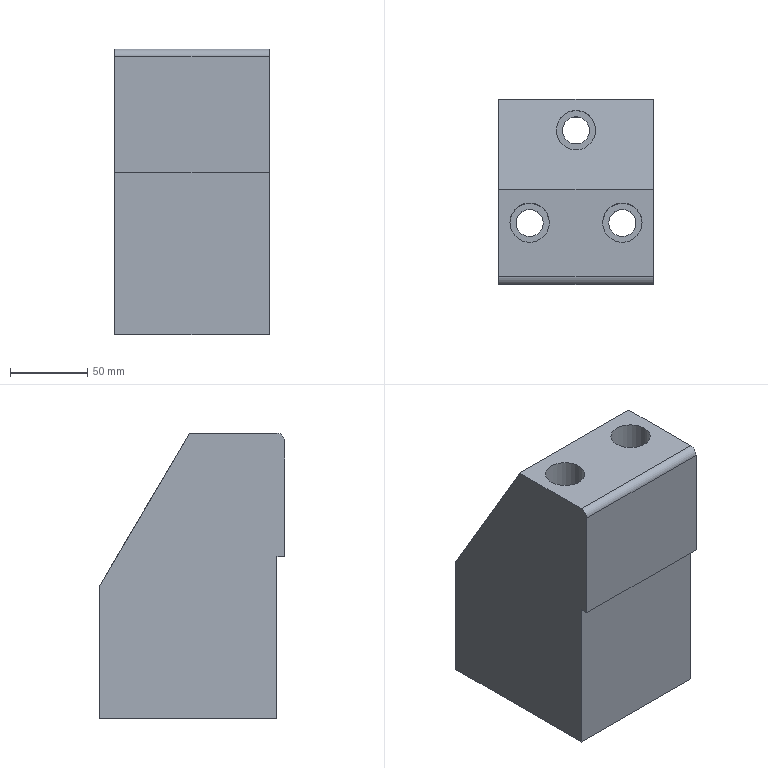Part | NX | features solid 2 | 1 solid | 19 faces | box 100 x 120 x 185 mm | volume 1651296 mm3 | plane 12 | cylinder 7 | commonest cylinder face diameters 17.5 x3 25.5 x3 10 x1
STEP:
#1=CARTESIAN_POINT('',(-412.5,235.,5.));
#2=VERTEX_POINT('',#1);
#3=CARTESIAN_POINT('',(-412.5,291.602,5.));
#4=VERTEX_POINT('',#3);
#5=CARTESIAN_POINT('',(-412.5,230.,5.));
#6=DIRECTION('',(0.,1.,0.));
#7=VECTOR('',#6,1000.);
#8=LINE('',#5,#7);
#9=EDGE_CURVE('',#2,#4,#8,.T.);
#10=ORIENTED_EDGE('',*,*,#9,.F.);
#11=CARTESIAN_POINT('',(-412.5,230.,0.));
#12=VERTEX_POINT('',#11);
#13=CARTESIAN_POINT('',(-412.5,235.,0.));
#14=DIRECTION('',(-1.,0.,0.));
#15=DIRECTION('',(0.,0.,1.));
#16=AXIS2_PLACEMENT_3D('',#13,#14,#15);
#17=CIRCLE('',#16,5.);
#18=EDGE_CURVE('',#2,#12,#17,.F.);
#19=ORIENTED_EDGE('',*,*,#18,.T.);
#20=CARTESIAN_POINT('',(-412.5,230.,-75.));
#21=VERTEX_POINT('',#20);
#22=CARTESIAN_POINT('',(-412.5,230.,-75.));
#23=DIRECTION('',(0.,0.,1.));
#24=VECTOR('',#23,1000.);
#25=LINE('',#22,#24);
#26=EDGE_CURVE('',#21,#12,#25,.T.);
#27=ORIENTED_EDGE('',*,*,#26,.F.);
#28=CARTESIAN_POINT('',(-412.5,235.,-75.));
#29=VERTEX_POINT('',#28);
#30=CARTESIAN_POINT('',(-412.5,230.,-75.));
#31=DIRECTION('',(0.,-1.,0.));
#32=VECTOR('',#31,1000.);
#33=LINE('',#30,#32);
#34=EDGE_CURVE('',#21,#29,#33,.F.);
#35=ORIENTED_EDGE('',*,*,#34,.T.);
#36=CARTESIAN_POINT('',(-412.5,235.,-180.));
#37=VERTEX_POINT('',#36);
#38=CARTESIAN_POINT('',(-412.5,235.,-75.));
#39=DIRECTION('',(0.,0.,-1.));
#40=VECTOR('',#39,1000.);
#41=LINE('',#38,#40);
#42=EDGE_CURVE('',#29,#37,#41,.T.);
#43=ORIENTED_EDGE('',*,*,#42,.T.);
#44=CARTESIAN_POINT('',(-412.5,350.,-180.));
#45=VERTEX_POINT('',#44);
#46=CARTESIAN_POINT('',(-412.5,230.,-180.));
#47=DIRECTION('',(0.,1.,0.));
#48=VECTOR('',#47,1000.);
#49=LINE('',#46,#48);
#50=EDGE_CURVE('',#37,#45,#49,.T.);
#51=ORIENTED_EDGE('',*,*,#50,.T.);
#52=CARTESIAN_POINT('',(-412.5,350.,-94.277));
#53=VERTEX_POINT('',#52);
#54=CARTESIAN_POINT('',(-412.5,350.,-75.));
#55=DIRECTION('',(0.,0.,1.));
#56=VECTOR('',#55,1000.);
#57=LINE('',#54,#56);
#58=EDGE_CURVE('',#45,#53,#57,.T.);
#59=ORIENTED_EDGE('',*,*,#58,.T.);
#60=CARTESIAN_POINT('',(-412.5,310.727,-27.513));
#61=DIRECTION('',(0.,-0.507,0.8619));
#62=VECTOR('',#61,1000.);
#63=LINE('',#60,#62);
#64=EDGE_CURVE('',#53,#4,#63,.T.);
#65=ORIENTED_EDGE('',*,*,#64,.T.);
#66=EDGE_LOOP('',(#10,#19,#27,#35,#43,#51,#59,#65));
#67=FACE_BOUND('',#66,.T.);
#68=CARTESIAN_POINT('',(-412.5,230.,-75.));
#69=DIRECTION('',(-1.,0.,0.));
#70=DIRECTION('',(0.,0.,1.));
#71=AXIS2_PLACEMENT_3D('',#68,#69,#70);
#72=PLANE('',#71);
#73=ADVANCED_FACE('',(#67),#72,.F.);
#74=CARTESIAN_POINT('',(-423.75,270.,-180.));
#75=VERTEX_POINT('',#74);
#76=CARTESIAN_POINT('',(-432.5,270.,-180.));
#77=DIRECTION('',(0.,0.,1.));
#78=DIRECTION('',(1.,0.,0.));
#79=AXIS2_PLACEMENT_3D('',#76,#77,#78);
#80=CIRCLE('',#79,8.75);
#81=EDGE_CURVE('',#75,#75,#80,.T.);
#82=ORIENTED_EDGE('',*,*,#81,.T.);
#83=EDGE_LOOP('',(#82));
#84=FACE_BOUND('',#83,.T.);
#85=CARTESIAN_POINT('',(-483.75,270.,-180.));
#86=VERTEX_POINT('',#85);
#87=CARTESIAN_POINT('',(-492.5,270.,-180.));
#88=DIRECTION('',(0.,0.,1.));
#89=DIRECTION('',(1.,0.,0.));
#90=AXIS2_PLACEMENT_3D('',#87,#88,#89);
#91=CIRCLE('',#90,8.75);
#92=EDGE_CURVE('',#86,#86,#91,.T.);
#93=ORIENTED_EDGE('',*,*,#92,.T.);
#94=EDGE_LOOP('',(#93));
#95=FACE_BOUND('',#94,.T.);
#96=CARTESIAN_POINT('',(-453.75,330.,-180.));
#97=VERTEX_POINT('',#96);
#98=CARTESIAN_POINT('',(-462.5,330.,-180.));
#99=DIRECTION('',(0.,0.,1.));
#100=DIRECTION('',(1.,0.,0.));
#101=AXIS2_PLACEMENT_3D('',#98,#99,#100);
#102=CIRCLE('',#101,8.75);
#103=EDGE_CURVE('',#97,#97,#102,.T.);
#104=ORIENTED_EDGE('',*,*,#103,.T.);
#105=EDGE_LOOP('',(#104));
#106=FACE_BOUND('',#105,.T.);
#107=CARTESIAN_POINT('',(-512.5,235.,-180.));
#108=VERTEX_POINT('',#107);
#109=CARTESIAN_POINT('',(-487.5,235.,-180.));
#110=DIRECTION('',(1.,0.,0.));
#111=VECTOR('',#110,1000.);
#112=LINE('',#109,#111);
#113=EDGE_CURVE('',#108,#37,#112,.T.);
#114=ORIENTED_EDGE('',*,*,#113,.F.);
#115=CARTESIAN_POINT('',(-512.5,350.,-180.));
#116=VERTEX_POINT('',#115);
#117=CARTESIAN_POINT('',(-512.5,230.,-180.));
#118=DIRECTION('',(0.,1.,0.));
#119=VECTOR('',#118,1000.);
#120=LINE('',#117,#119);
#121=EDGE_CURVE('',#108,#116,#120,.T.);
#122=ORIENTED_EDGE('',*,*,#121,.T.);
#123=CARTESIAN_POINT('',(-487.5,350.,-180.));
#124=DIRECTION('',(1.,0.,0.));
#125=VECTOR('',#124,1000.);
#126=LINE('',#123,#125);
#127=EDGE_CURVE('',#116,#45,#126,.T.);
#128=ORIENTED_EDGE('',*,*,#127,.T.);
#129=ORIENTED_EDGE('',*,*,#50,.F.);
#130=EDGE_LOOP('',(#114,#122,#128,#129));
#131=FACE_BOUND('',#130,.T.);
#132=CARTESIAN_POINT('',(-487.5,230.,-180.));
#133=DIRECTION('',(0.,0.,1.));
#134=DIRECTION('',(1.,0.,0.));
#135=AXIS2_PLACEMENT_3D('',#132,#133,#134);
#136=PLANE('',#135);
#137=ADVANCED_FACE('',(#84,#95,#106,#131),#136,.F.);
#138=CARTESIAN_POINT('',(-512.5,230.,0.));
#139=VERTEX_POINT('',#138);
#140=CARTESIAN_POINT('',(-512.5,230.,-75.));
#141=VERTEX_POINT('',#140);
#142=CARTESIAN_POINT('',(-512.5,230.,25.));
#143=DIRECTION('',(0.,0.,1.));
#144=VECTOR('',#143,1000.);
#145=LINE('',#142,#144);
#146=EDGE_CURVE('',#139,#141,#145,.F.);
#147=ORIENTED_EDGE('',*,*,#146,.F.);
#148=CARTESIAN_POINT('',(-512.5,235.,5.));
#149=VERTEX_POINT('',#148);
#150=CARTESIAN_POINT('',(-512.5,235.,0.));
#151=DIRECTION('',(1.,0.,0.));
#152=DIRECTION('',(0.,0.,-1.));
#153=AXIS2_PLACEMENT_3D('',#150,#151,#152);
#154=CIRCLE('',#153,5.);
#155=EDGE_CURVE('',#139,#149,#154,.F.);
#156=ORIENTED_EDGE('',*,*,#155,.T.);
#157=CARTESIAN_POINT('',(-512.5,291.602,5.));
#158=VERTEX_POINT('',#157);
#159=CARTESIAN_POINT('',(-512.5,230.,5.));
#160=DIRECTION('',(0.,1.,0.));
#161=VECTOR('',#160,1000.);
#162=LINE('',#159,#161);
#163=EDGE_CURVE('',#149,#158,#162,.T.);
#164=ORIENTED_EDGE('',*,*,#163,.T.);
#165=CARTESIAN_POINT('',(-512.5,350.,-94.277));
#166=VERTEX_POINT('',#165);
#167=CARTESIAN_POINT('',(-512.5,267.026,46.78));
#168=DIRECTION('',(0.,0.507,-0.8619));
#169=VECTOR('',#168,1000.);
#170=LINE('',#167,#169);
#171=EDGE_CURVE('',#158,#166,#170,.T.);
#172=ORIENTED_EDGE('',*,*,#171,.T.);
#173=CARTESIAN_POINT('',(-512.5,350.,25.));
#174=DIRECTION('',(0.,0.,-1.));
#175=VECTOR('',#174,1000.);
#176=LINE('',#173,#175);
#177=EDGE_CURVE('',#166,#116,#176,.T.);
#178=ORIENTED_EDGE('',*,*,#177,.T.);
#179=ORIENTED_EDGE('',*,*,#121,.F.);
#180=CARTESIAN_POINT('',(-512.5,235.,-75.));
#181=VERTEX_POINT('',#180);
#182=CARTESIAN_POINT('',(-512.5,235.,-75.));
#183=DIRECTION('',(0.,0.,-1.));
#184=VECTOR('',#183,1000.);
#185=LINE('',#182,#184);
#186=EDGE_CURVE('',#181,#108,#185,.T.);
#187=ORIENTED_EDGE('',*,*,#186,.F.);
#188=CARTESIAN_POINT('',(-512.5,230.,-75.));
#189=DIRECTION('',(0.,-1.,0.));
#190=VECTOR('',#189,1000.);
#191=LINE('',#188,#190);
#192=EDGE_CURVE('',#141,#181,#191,.F.);
#193=ORIENTED_EDGE('',*,*,#192,.F.);
#194=EDGE_LOOP('',(#147,#156,#164,#172,#178,#179,#187,#193));
#195=FACE_BOUND('',#194,.T.);
#196=CARTESIAN_POINT('',(-512.5,230.,25.));
#197=DIRECTION('',(1.,0.,0.));
#198=DIRECTION('',(0.,0.,-1.));
#199=AXIS2_PLACEMENT_3D('',#196,#197,#198);
#200=PLANE('',#199);
#201=ADVANCED_FACE('',(#195),#200,.F.);
#202=ORIENTED_EDGE('',*,*,#26,.T.);
#203=CARTESIAN_POINT('',(-512.5,230.,0.));
#204=DIRECTION('',(-1.,0.,0.));
#205=VECTOR('',#204,1000.);
#206=LINE('',#203,#205);
#207=EDGE_CURVE('',#12,#139,#206,.T.);
#208=ORIENTED_EDGE('',*,*,#207,.T.);
#209=ORIENTED_EDGE('',*,*,#146,.T.);
#210=CARTESIAN_POINT('',(-487.5,230.,-75.));
#211=DIRECTION('',(-1.,0.,0.));
#212=VECTOR('',#211,1000.);
#213=LINE('',#210,#212);
#214=EDGE_CURVE('',#141,#21,#213,.F.);
#215=ORIENTED_EDGE('',*,*,#214,.T.);
#216=EDGE_LOOP('',(#202,#208,#209,#215));
#217=FACE_BOUND('',#216,.T.);
#218=CARTESIAN_POINT('',(-487.5,230.,25.));
#219=DIRECTION('',(0.,-1.,0.));
#220=DIRECTION('',(1.,0.,0.));
#221=AXIS2_PLACEMENT_3D('',#218,#219,#220);
#222=PLANE('',#221);
#223=ADVANCED_FACE('',(#217),#222,.T.);
#224=CARTESIAN_POINT('',(-445.25,270.,5.));
#225=VERTEX_POINT('',#224);
#226=CARTESIAN_POINT('',(-432.5,270.,5.));
#227=DIRECTION('',(0.,0.,-1.));
#228=DIRECTION('',(-1.,0.,0.));
#229=AXIS2_PLACEMENT_3D('',#226,#227,#228);
#230=CIRCLE('',#229,12.75);
#231=EDGE_CURVE('',#225,#225,#230,.T.);
#232=ORIENTED_EDGE('',*,*,#231,.T.);
#233=EDGE_LOOP('',(#232));
#234=FACE_BOUND('',#233,.T.);
#235=CARTESIAN_POINT('',(-505.25,270.,5.));
#236=VERTEX_POINT('',#235);
#237=CARTESIAN_POINT('',(-492.5,270.,5.));
#238=DIRECTION('',(0.,0.,-1.));
#239=DIRECTION('',(-1.,0.,0.));
#240=AXIS2_PLACEMENT_3D('',#237,#238,#239);
#241=CIRCLE('',#240,12.75);
#242=EDGE_CURVE('',#236,#236,#241,.T.);
#243=ORIENTED_EDGE('',*,*,#242,.T.);
#244=EDGE_LOOP('',(#243));
#245=FACE_BOUND('',#244,.T.);
#246=ORIENTED_EDGE('',*,*,#163,.F.);
#247=CARTESIAN_POINT('',(-412.5,235.,5.));
#248=DIRECTION('',(-1.,0.,0.));
#249=VECTOR('',#248,1000.);
#250=LINE('',#247,#249);
#251=EDGE_CURVE('',#149,#2,#250,.F.);
#252=ORIENTED_EDGE('',*,*,#251,.T.);
#253=ORIENTED_EDGE('',*,*,#9,.T.);
#254=CARTESIAN_POINT('',(-412.5,291.602,5.));
#255=DIRECTION('',(-1.,0.,0.));
#256=VECTOR('',#255,1000.);
#257=LINE('',#254,#256);
#258=EDGE_CURVE('',#4,#158,#257,.T.);
#259=ORIENTED_EDGE('',*,*,#258,.T.);
#260=EDGE_LOOP('',(#246,#252,#253,#259));
#261=FACE_BOUND('',#260,.T.);
#262=CARTESIAN_POINT('',(-412.5,230.,5.));
#263=DIRECTION('',(0.,0.,-1.));
#264=DIRECTION('',(-1.,0.,0.));
#265=AXIS2_PLACEMENT_3D('',#262,#263,#264);
#266=PLANE('',#265);
#267=ADVANCED_FACE('',(#234,#245,#261),#266,.F.);
#268=ORIENTED_EDGE('',*,*,#177,.F.);
#269=CARTESIAN_POINT('',(-487.5,350.,-94.277));
#270=DIRECTION('',(1.,0.,0.));
#271=VECTOR('',#270,1000.);
#272=LINE('',#269,#271);
#273=EDGE_CURVE('',#166,#53,#272,.T.);
#274=ORIENTED_EDGE('',*,*,#273,.T.);
#275=ORIENTED_EDGE('',*,*,#58,.F.);
#276=ORIENTED_EDGE('',*,*,#127,.F.);
#277=EDGE_LOOP('',(#268,#274,#275,#276));
#278=FACE_BOUND('',#277,.T.);
#279=CARTESIAN_POINT('',(-487.5,350.,25.));
#280=DIRECTION('',(0.,-1.,0.));
#281=DIRECTION('',(1.,0.,0.));
#282=AXIS2_PLACEMENT_3D('',#279,#280,#281);
#283=PLANE('',#282);
#284=ADVANCED_FACE('',(#278),#283,.F.);
#285=CARTESIAN_POINT('',(-462.5,342.75,-81.952));
#286=VERTEX_POINT('',#285);
#287=CARTESIAN_POINT('',(-462.5,330.,-60.277));
#288=DIRECTION('',(0.,-0.8619,-0.507));
#289=DIRECTION('',(0.,0.507,-0.8619));
#290=AXIS2_PLACEMENT_3D('',#287,#288,#289);
#291=ELLIPSE('',#290,25.147,12.75);
#292=EDGE_CURVE('',#286,#286,#291,.T.);
#293=ORIENTED_EDGE('',*,*,#292,.T.);
#294=EDGE_LOOP('',(#293));
#295=FACE_BOUND('',#294,.T.);
#296=ORIENTED_EDGE('',*,*,#258,.F.);
#297=ORIENTED_EDGE('',*,*,#64,.F.);
#298=ORIENTED_EDGE('',*,*,#273,.F.);
#299=ORIENTED_EDGE('',*,*,#171,.F.);
#300=EDGE_LOOP('',(#296,#297,#298,#299));
#301=FACE_BOUND('',#300,.T.);
#302=CARTESIAN_POINT('',(-412.5,288.619,10.07));
#303=DIRECTION('',(0.,-0.8619,-0.507));
#304=DIRECTION('',(0.,0.507,-0.8619));
#305=AXIS2_PLACEMENT_3D('',#302,#303,#304);
#306=PLANE('',#305);
#307=ADVANCED_FACE('',(#295,#301),#306,.F.);
#308=CARTESIAN_POINT('',(-441.25,270.,-150.));
#309=VERTEX_POINT('',#308);
#310=CARTESIAN_POINT('',(-432.5,270.,-150.));
#311=DIRECTION('',(0.,0.,-1.));
#312=DIRECTION('',(-1.,0.,0.));
#313=AXIS2_PLACEMENT_3D('',#310,#311,#312);
#314=CIRCLE('',#313,8.75);
#315=EDGE_CURVE('',#309,#309,#314,.T.);
#316=ORIENTED_EDGE('',*,*,#315,.F.);
#317=EDGE_LOOP('',(#316));
#318=FACE_BOUND('',#317,.T.);
#319=ORIENTED_EDGE('',*,*,#81,.F.);
#320=EDGE_LOOP('',(#319));
#321=FACE_BOUND('',#320,.T.);
#322=CARTESIAN_POINT('',(-432.5,270.,-200.));
#323=DIRECTION('',(0.,0.,-1.));
#324=DIRECTION('',(-1.,0.,0.));
#325=AXIS2_PLACEMENT_3D('',#322,#323,#324);
#326=CYLINDRICAL_SURFACE('',#325,8.75);
#327=ADVANCED_FACE('',(#318,#321),#326,.F.);
#328=ORIENTED_EDGE('',*,*,#315,.T.);
#329=EDGE_LOOP('',(#328));
#330=FACE_BOUND('',#329,.T.);
#331=CARTESIAN_POINT('',(-445.25,270.,-150.));
#332=VERTEX_POINT('',#331);
#333=CARTESIAN_POINT('',(-432.5,270.,-150.));
#334=DIRECTION('',(0.,0.,-1.));
#335=DIRECTION('',(-1.,0.,0.));
#336=AXIS2_PLACEMENT_3D('',#333,#334,#335);
#337=CIRCLE('',#336,12.75);
#338=EDGE_CURVE('',#332,#332,#337,.T.);
#339=ORIENTED_EDGE('',*,*,#338,.F.);
#340=EDGE_LOOP('',(#339));
#341=FACE_BOUND('',#340,.T.);
#342=CARTESIAN_POINT('',(-432.5,265.,-150.));
#343=DIRECTION('',(0.,0.,-1.));
#344=DIRECTION('',(-1.,0.,0.));
#345=AXIS2_PLACEMENT_3D('',#342,#343,#344);
#346=PLANE('',#345);
#347=ADVANCED_FACE('',(#330,#341),#346,.F.);
#348=ORIENTED_EDGE('',*,*,#231,.F.);
#349=EDGE_LOOP('',(#348));
#350=FACE_BOUND('',#349,.T.);
#351=ORIENTED_EDGE('',*,*,#338,.T.);
#352=EDGE_LOOP('',(#351));
#353=FACE_BOUND('',#352,.T.);
#354=CARTESIAN_POINT('',(-432.5,270.,0.));
#355=DIRECTION('',(0.,0.,-1.));
#356=DIRECTION('',(-1.,0.,0.));
#357=AXIS2_PLACEMENT_3D('',#354,#355,#356);
#358=CYLINDRICAL_SURFACE('',#357,12.75);
#359=ADVANCED_FACE('',(#350,#353),#358,.F.);
#360=CARTESIAN_POINT('',(-501.25,270.,-150.));
#361=VERTEX_POINT('',#360);
#362=CARTESIAN_POINT('',(-492.5,270.,-150.));
#363=DIRECTION('',(0.,0.,-1.));
#364=DIRECTION('',(-1.,0.,0.));
#365=AXIS2_PLACEMENT_3D('',#362,#363,#364);
#366=CIRCLE('',#365,8.75);
#367=EDGE_CURVE('',#361,#361,#366,.T.);
#368=ORIENTED_EDGE('',*,*,#367,.F.);
#369=EDGE_LOOP('',(#368));
#370=FACE_BOUND('',#369,.T.);
#371=ORIENTED_EDGE('',*,*,#92,.F.);
#372=EDGE_LOOP('',(#371));
#373=FACE_BOUND('',#372,.T.);
#374=CARTESIAN_POINT('',(-492.5,270.,-200.));
#375=DIRECTION('',(0.,0.,-1.));
#376=DIRECTION('',(-1.,0.,0.));
#377=AXIS2_PLACEMENT_3D('',#374,#375,#376);
#378=CYLINDRICAL_SURFACE('',#377,8.75);
#379=ADVANCED_FACE('',(#370,#373),#378,.F.);
#380=ORIENTED_EDGE('',*,*,#367,.T.);
#381=EDGE_LOOP('',(#380));
#382=FACE_BOUND('',#381,.T.);
#383=CARTESIAN_POINT('',(-505.25,270.,-150.));
#384=VERTEX_POINT('',#383);
#385=CARTESIAN_POINT('',(-492.5,270.,-150.));
#386=DIRECTION('',(0.,0.,-1.));
#387=DIRECTION('',(-1.,0.,0.));
#388=AXIS2_PLACEMENT_3D('',#385,#386,#387);
#389=CIRCLE('',#388,12.75);
#390=EDGE_CURVE('',#384,#384,#389,.T.);
#391=ORIENTED_EDGE('',*,*,#390,.F.);
#392=EDGE_LOOP('',(#391));
#393=FACE_BOUND('',#392,.T.);
#394=CARTESIAN_POINT('',(-492.5,265.,-150.));
#395=DIRECTION('',(0.,0.,-1.));
#396=DIRECTION('',(-1.,0.,0.));
#397=AXIS2_PLACEMENT_3D('',#394,#395,#396);
#398=PLANE('',#397);
#399=ADVANCED_FACE('',(#382,#393),#398,.F.);
#400=ORIENTED_EDGE('',*,*,#242,.F.);
#401=EDGE_LOOP('',(#400));
#402=FACE_BOUND('',#401,.T.);
#403=ORIENTED_EDGE('',*,*,#390,.T.);
#404=EDGE_LOOP('',(#403));
#405=FACE_BOUND('',#404,.T.);
#406=CARTESIAN_POINT('',(-492.5,270.,0.));
#407=DIRECTION('',(0.,0.,-1.));
#408=DIRECTION('',(-1.,0.,0.));
#409=AXIS2_PLACEMENT_3D('',#406,#407,#408);
#410=CYLINDRICAL_SURFACE('',#409,12.75);
#411=ADVANCED_FACE('',(#402,#405),#410,.F.);
#412=CARTESIAN_POINT('',(-471.25,330.,-150.));
#413=VERTEX_POINT('',#412);
#414=CARTESIAN_POINT('',(-462.5,330.,-150.));
#415=DIRECTION('',(0.,0.,-1.));
#416=DIRECTION('',(-1.,0.,0.));
#417=AXIS2_PLACEMENT_3D('',#414,#415,#416);
#418=CIRCLE('',#417,8.75);
#419=EDGE_CURVE('',#413,#413,#418,.T.);
#420=ORIENTED_EDGE('',*,*,#419,.F.);
#421=EDGE_LOOP('',(#420));
#422=FACE_BOUND('',#421,.T.);
#423=ORIENTED_EDGE('',*,*,#103,.F.);
#424=EDGE_LOOP('',(#423));
#425=FACE_BOUND('',#424,.T.);
#426=CARTESIAN_POINT('',(-462.5,330.,-200.));
#427=DIRECTION('',(0.,0.,-1.));
#428=DIRECTION('',(-1.,0.,0.));
#429=AXIS2_PLACEMENT_3D('',#426,#427,#428);
#430=CYLINDRICAL_SURFACE('',#429,8.75);
#431=ADVANCED_FACE('',(#422,#425),#430,.F.);
#432=CARTESIAN_POINT('',(-475.25,330.,-150.));
#433=VERTEX_POINT('',#432);
#434=CARTESIAN_POINT('',(-462.5,330.,-150.));
#435=DIRECTION('',(0.,0.,-1.));
#436=DIRECTION('',(-1.,0.,0.));
#437=AXIS2_PLACEMENT_3D('',#434,#435,#436);
#438=CIRCLE('',#437,12.75);
#439=EDGE_CURVE('',#433,#433,#438,.T.);
#440=ORIENTED_EDGE('',*,*,#439,.T.);
#441=EDGE_LOOP('',(#440));
#442=FACE_BOUND('',#441,.T.);
#443=ORIENTED_EDGE('',*,*,#292,.F.);
#444=EDGE_LOOP('',(#443));
#445=FACE_BOUND('',#444,.T.);
#446=CARTESIAN_POINT('',(-462.5,330.,0.));
#447=DIRECTION('',(0.,0.,-1.));
#448=DIRECTION('',(-1.,0.,0.));
#449=AXIS2_PLACEMENT_3D('',#446,#447,#448);
#450=CYLINDRICAL_SURFACE('',#449,12.75);
#451=ADVANCED_FACE('',(#442,#445),#450,.F.);
#452=ORIENTED_EDGE('',*,*,#419,.T.);
#453=EDGE_LOOP('',(#452));
#454=FACE_BOUND('',#453,.T.);
#455=ORIENTED_EDGE('',*,*,#439,.F.);
#456=EDGE_LOOP('',(#455));
#457=FACE_BOUND('',#456,.T.);
#458=CARTESIAN_POINT('',(-462.5,330.,-150.));
#459=DIRECTION('',(0.,0.,-1.));
#460=DIRECTION('',(-1.,0.,0.));
#461=AXIS2_PLACEMENT_3D('',#458,#459,#460);
#462=PLANE('',#461);
#463=ADVANCED_FACE('',(#454,#457),#462,.F.);
#464=ORIENTED_EDGE('',*,*,#113,.T.);
#465=ORIENTED_EDGE('',*,*,#42,.F.);
#466=CARTESIAN_POINT('',(-412.5,235.,-75.));
#467=DIRECTION('',(1.,0.,0.));
#468=VECTOR('',#467,1000.);
#469=LINE('',#466,#468);
#470=EDGE_CURVE('',#29,#181,#469,.F.);
#471=ORIENTED_EDGE('',*,*,#470,.T.);
#472=ORIENTED_EDGE('',*,*,#186,.T.);
#473=EDGE_LOOP('',(#464,#465,#471,#472));
#474=FACE_BOUND('',#473,.T.);
#475=CARTESIAN_POINT('',(-412.5,235.,-75.));
#476=DIRECTION('',(0.,-1.,0.));
#477=DIRECTION('',(0.,0.,-1.));
#478=AXIS2_PLACEMENT_3D('',#475,#476,#477);
#479=PLANE('',#478);
#480=ADVANCED_FACE('',(#474),#479,.T.);
#481=ORIENTED_EDGE('',*,*,#192,.T.);
#482=ORIENTED_EDGE('',*,*,#470,.F.);
#483=ORIENTED_EDGE('',*,*,#34,.F.);
#484=ORIENTED_EDGE('',*,*,#214,.F.);
#485=EDGE_LOOP('',(#481,#482,#483,#484));
#486=FACE_BOUND('',#485,.T.);
#487=CARTESIAN_POINT('',(-412.5,230.,-75.));
#488=DIRECTION('',(0.,0.,1.));
#489=DIRECTION('',(-1.,0.,0.));
#490=AXIS2_PLACEMENT_3D('',#487,#488,#489);
#491=PLANE('',#490);
#492=ADVANCED_FACE('',(#486),#491,.F.);
#493=ORIENTED_EDGE('',*,*,#18,.F.);
#494=ORIENTED_EDGE('',*,*,#251,.F.);
#495=ORIENTED_EDGE('',*,*,#155,.F.);
#496=ORIENTED_EDGE('',*,*,#207,.F.);
#497=EDGE_LOOP('',(#493,#494,#495,#496));
#498=FACE_BOUND('',#497,.T.);
#499=CARTESIAN_POINT('',(-487.5,235.,0.));
#500=DIRECTION('',(1.,0.,0.));
#501=DIRECTION('',(0.,0.,-1.));
#502=AXIS2_PLACEMENT_3D('',#499,#500,#501);
#503=CYLINDRICAL_SURFACE('',#502,5.);
#504=ADVANCED_FACE('',(#498),#503,.T.);
#505=CLOSED_SHELL('',(#73,#137,#201,#223,#267,#284,#307,#327,#347,#359,#379,#399,#411,#431,#451,#463,#480,#492,#504));
#506=MANIFOLD_SOLID_BREP('',#505);
#507=(LENGTH_UNIT()NAMED_UNIT(*)SI_UNIT(.MILLI.,.METRE.));
#508=UNCERTAINTY_MEASURE_WITH_UNIT(LENGTH_MEASURE(0.00001),#507,'','');
#509=(NAMED_UNIT(*)PLANE_ANGLE_UNIT()SI_UNIT($,.RADIAN.));
#510=(NAMED_UNIT(*)SI_UNIT($,.STERADIAN.)SOLID_ANGLE_UNIT());
#511=(GEOMETRIC_REPRESENTATION_CONTEXT(3)GLOBAL_UNCERTAINTY_ASSIGNED_CONTEXT((#508))GLOBAL_UNIT_ASSIGNED_CONTEXT((#507,#509,#510))REPRESENTATION_CONTEXT('',''));
#512=ADVANCED_BREP_SHAPE_REPRESENTATION('',(#506),#511);